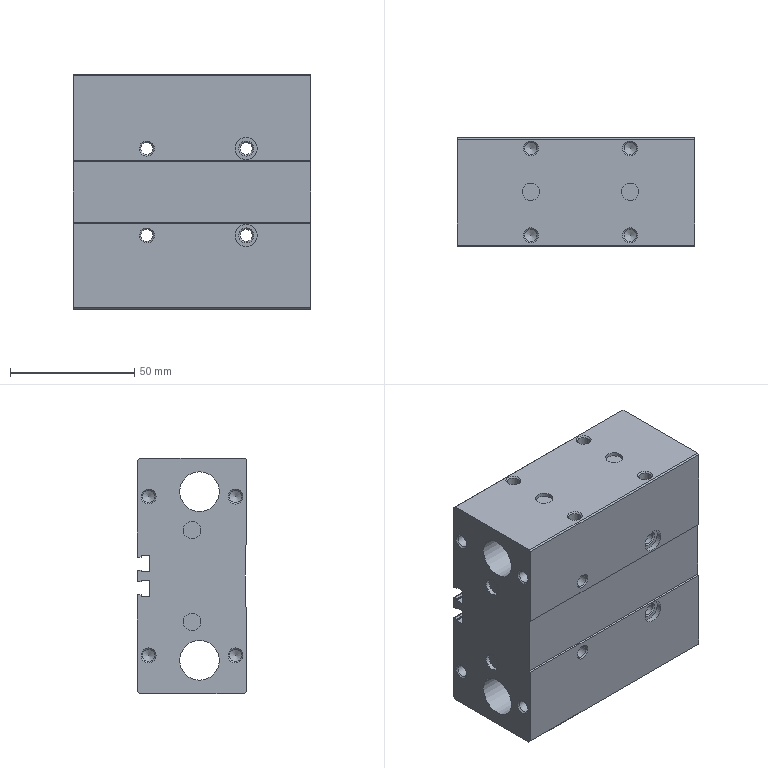Part | NX | features BREP 1 | 1 solid | 126 faces | box 95.6 x 44.05 x 95 mm | volume 307900 mm3 | plane 51 | cylinder 51 | cone 24 | commonest cylinder face diameters 4.917 x12 0.4 x8 0.8 x8 9 x6 5.2 x4 7 x4